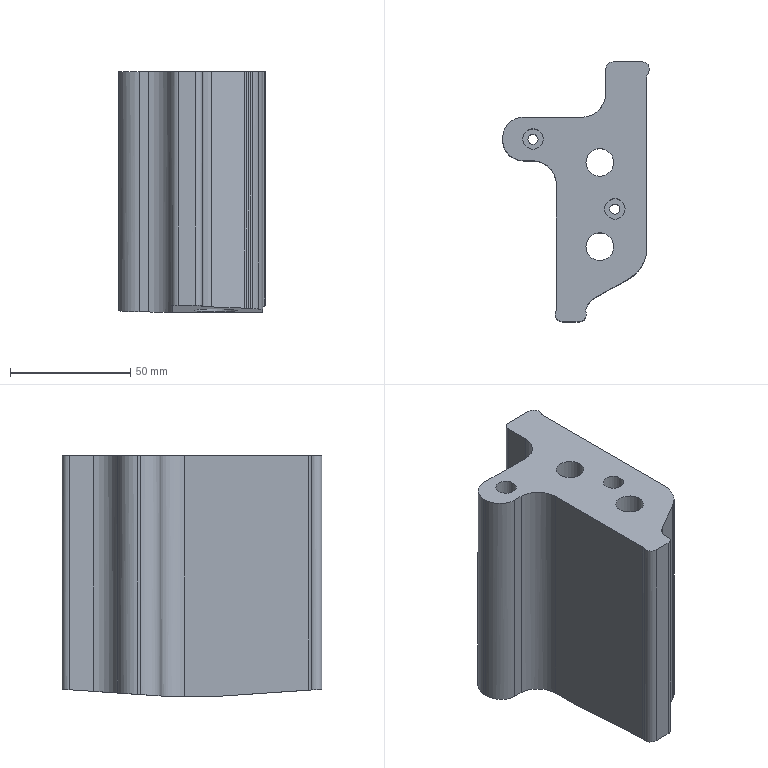Part | STEP file | lll_id250_x_t | 1 solid | 48 faces | box 60.865 x 107.859 x 100.003 mm | volume 310408 mm3 | cylinder 29 | plane 18 | cone 1 | commonest cylinder face diameters 6 x7 4.2 x2 8.506 x2 11.5 x2 17.001 x2 18.008 x2
STEP:
#1=CARTESIAN_POINT('',(449.,-109.43,-7.5));
#2=VERTEX_POINT('',#1);
#3=CARTESIAN_POINT('',(449.,-96.5,-7.5));
#4=VERTEX_POINT('',#3);
#5=CARTESIAN_POINT('',(449.,48.5,-7.5));
#6=DIRECTION('',(0.,1.,0.));
#7=VECTOR('',#6,1.);
#8=LINE('',#5,#7);
#9=EDGE_CURVE('',#2,#4,#8,.T.);
#10=ORIENTED_EDGE('',*,*,#9,.T.);
#11=CARTESIAN_POINT('',(446.115,-89.474,-7.502));
#12=VERTEX_POINT('',#11);
#13=CARTESIAN_POINT('',(438.999,-96.501,-7.5));
#14=DIRECTION('',(0.,0.,1.));
#15=DIRECTION('',(-1.,0.,0.));
#16=AXIS2_PLACEMENT_3D('',#13,#14,#15);
#17=CIRCLE('',#16,10.001);
#18=EDGE_CURVE('',#4,#12,#17,.T.);
#19=ORIENTED_EDGE('',*,*,#18,.T.);
#20=CARTESIAN_POINT('',(458.269,-89.43,-7.5));
#21=VERTEX_POINT('',#20);
#22=CARTESIAN_POINT('',(458.269,-89.43,-7.5));
#23=CARTESIAN_POINT('',(454.218,-89.444,-7.501));
#24=CARTESIAN_POINT('',(450.166,-89.459,-7.502));
#25=CARTESIAN_POINT('',(446.115,-89.474,-7.503));
#26=B_SPLINE_CURVE_WITH_KNOTS('',3,(#22,#23,#24,#25),.UNSPECIFIED.,.F.,.F.,(4,4),(0.,1.),.UNSPECIFIED.);
#27=EDGE_CURVE('',#21,#12,#26,.T.);
#28=ORIENTED_EDGE('',*,*,#27,.F.);
#29=CARTESIAN_POINT('',(475.731,-89.43,-7.5));
#30=VERTEX_POINT('',#29);
#31=CARTESIAN_POINT('',(467.,-87.231,-7.5));
#32=DIRECTION('',(0.,0.,-1.));
#33=DIRECTION('',(-1.,0.,0.));
#34=AXIS2_PLACEMENT_3D('',#31,#32,#33);
#35=CIRCLE('',#34,9.004);
#36=EDGE_CURVE('',#30,#21,#35,.T.);
#37=ORIENTED_EDGE('',*,*,#36,.F.);
#38=CARTESIAN_POINT('',(486.508,-89.43,-7.5));
#39=VERTEX_POINT('',#38);
#40=CARTESIAN_POINT('',(781.007,-89.43,-7.5));
#41=DIRECTION('',(-1.,0.,0.));
#42=VECTOR('',#41,1.);
#43=LINE('',#40,#42);
#44=EDGE_CURVE('',#39,#30,#43,.T.);
#45=ORIENTED_EDGE('',*,*,#44,.F.);
#46=CARTESIAN_POINT('',(486.507,-109.43,-7.5));
#47=VERTEX_POINT('',#46);
#48=CARTESIAN_POINT('',(486.516,48.518,-7.5));
#49=DIRECTION('',(-0.00006142,-1.,0.));
#50=VECTOR('',#49,1.);
#51=LINE('',#48,#50);
#52=EDGE_CURVE('',#39,#47,#51,.T.);
#53=ORIENTED_EDGE('',*,*,#52,.T.);
#54=CARTESIAN_POINT('',(465.982,-109.43,-7.5));
#55=VERTEX_POINT('',#54);
#56=CARTESIAN_POINT('',(488.085,-109.43,-7.5));
#57=DIRECTION('',(1.,0.,0.));
#58=VECTOR('',#57,1.);
#59=LINE('',#56,#58);
#60=EDGE_CURVE('',#55,#47,#59,.T.);
#61=ORIENTED_EDGE('',*,*,#60,.F.);
#62=CARTESIAN_POINT('',(458.045,-109.43,-7.5));
#63=VERTEX_POINT('',#62);
#64=CARTESIAN_POINT('',(462.014,-104.93,-7.5));
#65=DIRECTION('',(0.,0.,-1.));
#66=DIRECTION('',(-1.,0.,0.));
#67=AXIS2_PLACEMENT_3D('',#64,#65,#66);
#68=CIRCLE('',#67,6.);
#69=EDGE_CURVE('',#63,#55,#68,.T.);
#70=ORIENTED_EDGE('',*,*,#69,.F.);
#71=CARTESIAN_POINT('',(488.085,-109.43,-7.5));
#72=DIRECTION('',(1.,0.,0.));
#73=VECTOR('',#72,1.);
#74=LINE('',#71,#73);
#75=EDGE_CURVE('',#2,#63,#74,.T.);
#76=ORIENTED_EDGE('',*,*,#75,.F.);
#77=EDGE_LOOP('',(#10,#19,#28,#37,#45,#53,#61,#70,#76));
#78=FACE_BOUND('',#77,.T.);
#79=CARTESIAN_POINT('',(471.165,-106.5,-7.5));
#80=VERTEX_POINT('',#79);
#81=CARTESIAN_POINT('',(473.265,-106.5,-7.5));
#82=DIRECTION('',(0.,0.,1.));
#83=DIRECTION('',(-1.,0.,0.));
#84=AXIS2_PLACEMENT_3D('',#81,#82,#83);
#85=CIRCLE('',#84,2.1);
#86=EDGE_CURVE('',#80,#80,#85,.T.);
#87=ORIENTED_EDGE('',*,*,#86,.T.);
#88=EDGE_LOOP('',(#87));
#89=FACE_BOUND('',#88,.T.);
#90=CARTESIAN_POINT('',(781.007,48.5,-7.5));
#91=DIRECTION('',(0.,0.,-1.));
#92=DIRECTION('',(1.,0.,0.));
#93=AXIS2_PLACEMENT_3D('',#90,#91,#92);
#94=PLANE('',#93);
#95=ADVANCED_FACE('',(#78,#89),#94,.T.);
#96=CARTESIAN_POINT('',(476.004,-122.231,44.5));
#97=VERTEX_POINT('',#96);
#98=CARTESIAN_POINT('',(467.,-122.231,44.5));
#99=DIRECTION('',(0.,0.,-1.));
#100=DIRECTION('',(1.,0.,0.));
#101=AXIS2_PLACEMENT_3D('',#98,#99,#100);
#102=CIRCLE('',#101,9.004);
#103=EDGE_CURVE('',#97,#97,#102,.T.);
#104=ORIENTED_EDGE('',*,*,#103,.F.);
#105=EDGE_LOOP('',(#104));
#106=FACE_BOUND('',#105,.T.);
#107=CARTESIAN_POINT('',(467.,-131.235,-6.011));
#108=VERTEX_POINT('',#107);
#109=CARTESIAN_POINT('',(467.,-122.231,-6.626));
#110=DIRECTION('',(0.,-0.06813,-0.9977));
#111=DIRECTION('',(0.,-0.9977,0.06813));
#112=AXIS2_PLACEMENT_3D('',#109,#110,#111);
#113=ELLIPSE('',#112,9.025,9.004);
#114=EDGE_CURVE('',#108,#108,#113,.T.);
#115=ORIENTED_EDGE('',*,*,#114,.T.);
#116=EDGE_LOOP('',(#115));
#117=FACE_BOUND('',#116,.T.);
#118=CARTESIAN_POINT('',(467.,-122.231,-5.5));
#119=DIRECTION('',(0.,0.,1.));
#120=DIRECTION('',(1.,0.,0.));
#121=AXIS2_PLACEMENT_3D('',#118,#119,#120);
#122=CYLINDRICAL_SURFACE('',#121,9.004);
#123=ADVANCED_FACE('',(#106,#117),#122,.F.);
#124=CARTESIAN_POINT('',(468.014,-104.93,-2.296));
#125=VERTEX_POINT('',#124);
#126=CARTESIAN_POINT('',(462.014,-104.93,-2.296));
#127=DIRECTION('',(0.,0.,1.));
#128=DIRECTION('',(1.,0.,0.));
#129=AXIS2_PLACEMENT_3D('',#126,#127,#128);
#130=CIRCLE('',#129,6.);
#131=EDGE_CURVE('',#125,#125,#130,.T.);
#132=ORIENTED_EDGE('',*,*,#131,.T.);
#133=EDGE_LOOP('',(#132));
#134=FACE_BOUND('',#133,.T.);
#135=CARTESIAN_POINT('',(462.014,-104.93,-7.807));
#136=DIRECTION('',(0.,-0.06813,-0.9977));
#137=DIRECTION('',(0.,-0.9977,0.06813));
#138=AXIS2_PLACEMENT_3D('',#135,#136,#137);
#139=ELLIPSE('',#138,6.014,6.);
#140=EDGE_CURVE('',#55,#63,#139,.T.);
#141=ORIENTED_EDGE('',*,*,#140,.T.);
#142=ORIENTED_EDGE('',*,*,#69,.T.);
#143=EDGE_LOOP('',(#141,#142));
#144=FACE_BOUND('',#143,.T.);
#145=CARTESIAN_POINT('',(462.014,-104.93,-7.296));
#146=DIRECTION('',(0.,0.,1.));
#147=DIRECTION('',(-1.,0.,0.));
#148=AXIS2_PLACEMENT_3D('',#145,#146,#147);
#149=CYLINDRICAL_SURFACE('',#148,6.);
#150=ADVANCED_FACE('',(#134,#144),#149,.F.);
#151=ORIENTED_EDGE('',*,*,#103,.T.);
#152=EDGE_LOOP('',(#151));
#153=FACE_BOUND('',#152,.T.);
#154=CARTESIAN_POINT('',(472.75,-122.231,44.5));
#155=VERTEX_POINT('',#154);
#156=CARTESIAN_POINT('',(467.,-122.231,44.5));
#157=DIRECTION('',(0.,0.,1.));
#158=DIRECTION('',(1.,0.,0.));
#159=AXIS2_PLACEMENT_3D('',#156,#157,#158);
#160=CIRCLE('',#159,5.75);
#161=EDGE_CURVE('',#155,#155,#160,.T.);
#162=ORIENTED_EDGE('',*,*,#161,.T.);
#163=EDGE_LOOP('',(#162));
#164=FACE_BOUND('',#163,.T.);
#165=CARTESIAN_POINT('',(467.,-122.231,44.5));
#166=DIRECTION('',(0.,0.,1.));
#167=DIRECTION('',(1.,0.,0.));
#168=AXIS2_PLACEMENT_3D('',#165,#166,#167);
#169=PLANE('',#168);
#170=ADVANCED_FACE('',(#153,#164),#169,.F.);
#171=CARTESIAN_POINT('',(476.004,-87.231,44.5));
#172=VERTEX_POINT('',#171);
#173=CARTESIAN_POINT('',(467.,-87.231,44.5));
#174=DIRECTION('',(0.,0.,-1.));
#175=DIRECTION('',(1.,0.,0.));
#176=AXIS2_PLACEMENT_3D('',#173,#174,#175);
#177=CIRCLE('',#176,9.004);
#178=EDGE_CURVE('',#172,#172,#177,.T.);
#179=ORIENTED_EDGE('',*,*,#178,.T.);
#180=EDGE_LOOP('',(#179));
#181=FACE_BOUND('',#180,.T.);
#182=CARTESIAN_POINT('',(472.75,-87.231,44.5));
#183=VERTEX_POINT('',#182);
#184=CARTESIAN_POINT('',(467.,-87.231,44.5));
#185=DIRECTION('',(0.,0.,1.));
#186=DIRECTION('',(1.,0.,0.));
#187=AXIS2_PLACEMENT_3D('',#184,#185,#186);
#188=CIRCLE('',#187,5.75);
#189=EDGE_CURVE('',#183,#183,#188,.T.);
#190=ORIENTED_EDGE('',*,*,#189,.T.);
#191=EDGE_LOOP('',(#190));
#192=FACE_BOUND('',#191,.T.);
#193=CARTESIAN_POINT('',(467.,-87.231,44.5));
#194=DIRECTION('',(0.,0.,1.));
#195=DIRECTION('',(1.,0.,0.));
#196=AXIS2_PLACEMENT_3D('',#193,#194,#195);
#197=PLANE('',#196);
#198=ADVANCED_FACE('',(#181,#192),#197,.F.);
#199=CARTESIAN_POINT('',(469.012,-106.5,30.747));
#200=VERTEX_POINT('',#199);
#201=CARTESIAN_POINT('',(473.265,-106.5,30.747));
#202=DIRECTION('',(0.,0.,1.));
#203=DIRECTION('',(-1.,0.,0.));
#204=AXIS2_PLACEMENT_3D('',#201,#202,#203);
#205=CIRCLE('',#204,4.253);
#206=EDGE_CURVE('',#200,#200,#205,.T.);
#207=ORIENTED_EDGE('',*,*,#206,.F.);
#208=EDGE_LOOP('',(#207));
#209=FACE_BOUND('',#208,.T.);
#210=CARTESIAN_POINT('',(469.012,-106.5,92.5));
#211=VERTEX_POINT('',#210);
#212=CARTESIAN_POINT('',(473.265,-106.5,92.5));
#213=DIRECTION('',(0.,0.,-1.));
#214=DIRECTION('',(-1.,0.,0.));
#215=AXIS2_PLACEMENT_3D('',#212,#213,#214);
#216=CIRCLE('',#215,4.253);
#217=EDGE_CURVE('',#211,#211,#216,.T.);
#218=ORIENTED_EDGE('',*,*,#217,.F.);
#219=EDGE_LOOP('',(#218));
#220=FACE_BOUND('',#219,.T.);
#221=CARTESIAN_POINT('',(473.265,-106.5,180.747));
#222=DIRECTION('',(0.,0.,-1.));
#223=DIRECTION('',(1.,0.,0.));
#224=AXIS2_PLACEMENT_3D('',#221,#222,#223);
#225=CYLINDRICAL_SURFACE('',#224,4.253);
#226=ADVANCED_FACE('',(#209,#220),#225,.F.);
#227=CARTESIAN_POINT('',(435.012,-77.5,30.747));
#228=VERTEX_POINT('',#227);
#229=CARTESIAN_POINT('',(439.265,-77.5,30.747));
#230=DIRECTION('',(0.,0.,1.));
#231=DIRECTION('',(-1.,0.,0.));
#232=AXIS2_PLACEMENT_3D('',#229,#230,#231);
#233=CIRCLE('',#232,4.253);
#234=EDGE_CURVE('',#228,#228,#233,.T.);
#235=ORIENTED_EDGE('',*,*,#234,.F.);
#236=EDGE_LOOP('',(#235));
#237=FACE_BOUND('',#236,.T.);
#238=CARTESIAN_POINT('',(435.012,-77.5,92.5));
#239=VERTEX_POINT('',#238);
#240=CARTESIAN_POINT('',(439.265,-77.5,92.5));
#241=DIRECTION('',(0.,0.,-1.));
#242=DIRECTION('',(-1.,0.,0.));
#243=AXIS2_PLACEMENT_3D('',#240,#241,#242);
#244=CIRCLE('',#243,4.253);
#245=EDGE_CURVE('',#239,#239,#244,.T.);
#246=ORIENTED_EDGE('',*,*,#245,.F.);
#247=EDGE_LOOP('',(#246));
#248=FACE_BOUND('',#247,.T.);
#249=CARTESIAN_POINT('',(439.265,-77.5,180.747));
#250=DIRECTION('',(0.,0.,-1.));
#251=DIRECTION('',(1.,0.,0.));
#252=AXIS2_PLACEMENT_3D('',#249,#250,#251);
#253=CYLINDRICAL_SURFACE('',#252,4.253);
#254=ADVANCED_FACE('',(#237,#248),#253,.F.);
#255=CARTESIAN_POINT('',(471.165,-106.5,30.747));
#256=VERTEX_POINT('',#255);
#257=CARTESIAN_POINT('',(473.265,-106.5,30.747));
#258=DIRECTION('',(0.,0.,1.));
#259=DIRECTION('',(-1.,0.,0.));
#260=AXIS2_PLACEMENT_3D('',#257,#258,#259);
#261=CIRCLE('',#260,2.1);
#262=EDGE_CURVE('',#256,#256,#261,.T.);
#263=ORIENTED_EDGE('',*,*,#262,.F.);
#264=EDGE_LOOP('',(#263));
#265=FACE_BOUND('',#264,.T.);
#266=ORIENTED_EDGE('',*,*,#206,.T.);
#267=EDGE_LOOP('',(#266));
#268=FACE_BOUND('',#267,.T.);
#269=CARTESIAN_POINT('',(473.265,-106.5,30.747));
#270=DIRECTION('',(0.,0.,-1.));
#271=DIRECTION('',(1.,0.,0.));
#272=AXIS2_PLACEMENT_3D('',#269,#270,#271);
#273=PLANE('',#272);
#274=ADVANCED_FACE('',(#265,#268),#273,.F.);
#275=ORIENTED_EDGE('',*,*,#262,.T.);
#276=EDGE_LOOP('',(#275));
#277=FACE_BOUND('',#276,.T.);
#278=ORIENTED_EDGE('',*,*,#86,.F.);
#279=EDGE_LOOP('',(#278));
#280=FACE_BOUND('',#279,.T.);
#281=CARTESIAN_POINT('',(473.265,-106.5,1343.726));
#282=DIRECTION('',(0.,0.,-1.));
#283=DIRECTION('',(1.,0.,0.));
#284=AXIS2_PLACEMENT_3D('',#281,#282,#283);
#285=CYLINDRICAL_SURFACE('',#284,2.1);
#286=ADVANCED_FACE('',(#277,#280),#285,.F.);
#287=CARTESIAN_POINT('',(437.165,-77.5,30.747));
#288=VERTEX_POINT('',#287);
#289=CARTESIAN_POINT('',(439.265,-77.5,30.747));
#290=DIRECTION('',(0.,0.,1.));
#291=DIRECTION('',(-1.,0.,0.));
#292=AXIS2_PLACEMENT_3D('',#289,#290,#291);
#293=CIRCLE('',#292,2.1);
#294=EDGE_CURVE('',#288,#288,#293,.T.);
#295=ORIENTED_EDGE('',*,*,#294,.F.);
#296=EDGE_LOOP('',(#295));
#297=FACE_BOUND('',#296,.T.);
#298=ORIENTED_EDGE('',*,*,#234,.T.);
#299=EDGE_LOOP('',(#298));
#300=FACE_BOUND('',#299,.T.);
#301=CARTESIAN_POINT('',(439.265,-77.5,30.747));
#302=DIRECTION('',(0.,0.,-1.));
#303=DIRECTION('',(1.,0.,0.));
#304=AXIS2_PLACEMENT_3D('',#301,#302,#303);
#305=PLANE('',#304);
#306=ADVANCED_FACE('',(#297,#300),#305,.F.);
#307=CARTESIAN_POINT('',(439.265,-79.6,-6.829));
#308=VERTEX_POINT('',#307);
#309=CARTESIAN_POINT('',(439.265,-77.5,-6.685));
#310=DIRECTION('',(0.,-0.06813,0.9977));
#311=DIRECTION('',(0.,-0.9977,-0.06813));
#312=AXIS2_PLACEMENT_3D('',#309,#310,#311);
#313=ELLIPSE('',#312,2.105,2.1);
#314=EDGE_CURVE('',#308,#308,#313,.T.);
#315=ORIENTED_EDGE('',*,*,#314,.F.);
#316=EDGE_LOOP('',(#315));
#317=FACE_BOUND('',#316,.T.);
#318=ORIENTED_EDGE('',*,*,#294,.T.);
#319=EDGE_LOOP('',(#318));
#320=FACE_BOUND('',#319,.T.);
#321=CARTESIAN_POINT('',(439.265,-77.5,1343.726));
#322=DIRECTION('',(0.,0.,-1.));
#323=DIRECTION('',(1.,0.,0.));
#324=AXIS2_PLACEMENT_3D('',#321,#322,#323);
#325=CYLINDRICAL_SURFACE('',#324,2.1);
#326=ADVANCED_FACE('',(#317,#320),#325,.F.);
#327=ORIENTED_EDGE('',*,*,#36,.T.);
#328=CARTESIAN_POINT('',(467.,-87.231,-7.35));
#329=DIRECTION('',(0.,-0.06813,0.9977));
#330=DIRECTION('',(0.,0.9977,0.06813));
#331=AXIS2_PLACEMENT_3D('',#328,#329,#330);
#332=ELLIPSE('',#331,9.025,9.004);
#333=EDGE_CURVE('',#30,#21,#332,.T.);
#334=ORIENTED_EDGE('',*,*,#333,.F.);
#335=EDGE_LOOP('',(#327,#334));
#336=FACE_BOUND('',#335,.T.);
#337=ORIENTED_EDGE('',*,*,#178,.F.);
#338=EDGE_LOOP('',(#337));
#339=FACE_BOUND('',#338,.T.);
#340=CARTESIAN_POINT('',(467.,-87.231,-5.5));
#341=DIRECTION('',(0.,0.,1.));
#342=DIRECTION('',(1.,0.,0.));
#343=AXIS2_PLACEMENT_3D('',#340,#341,#342);
#344=CYLINDRICAL_SURFACE('',#343,9.004);
#345=ADVANCED_FACE('',(#336,#339),#344,.F.);
#346=ORIENTED_EDGE('',*,*,#161,.F.);
#347=EDGE_LOOP('',(#346));
#348=FACE_BOUND('',#347,.T.);
#349=CARTESIAN_POINT('',(461.25,-122.231,92.5));
#350=VERTEX_POINT('',#349);
#351=CARTESIAN_POINT('',(467.,-122.231,92.5));
#352=DIRECTION('',(0.,0.,-1.));
#353=DIRECTION('',(-1.,0.,0.));
#354=AXIS2_PLACEMENT_3D('',#351,#352,#353);
#355=CIRCLE('',#354,5.75);
#356=EDGE_CURVE('',#350,#350,#355,.T.);
#357=ORIENTED_EDGE('',*,*,#356,.F.);
#358=EDGE_LOOP('',(#357));
#359=FACE_BOUND('',#358,.T.);
#360=CARTESIAN_POINT('',(467.,-122.231,94.5));
#361=DIRECTION('',(0.,0.,-1.));
#362=DIRECTION('',(1.,0.,0.));
#363=AXIS2_PLACEMENT_3D('',#360,#361,#362);
#364=CYLINDRICAL_SURFACE('',#363,5.75);
#365=ADVANCED_FACE('',(#348,#359),#364,.F.);
#366=CARTESIAN_POINT('',(461.302,-149.551,92.5));
#367=VERTEX_POINT('',#366);
#368=CARTESIAN_POINT('',(461.369,-147.727,92.5));
#369=VERTEX_POINT('',#368);
#370=CARTESIAN_POINT('',(464.191,-148.744,92.5));
#371=DIRECTION('',(0.,0.,-1.));
#372=DIRECTION('',(-1.,0.,0.));
#373=AXIS2_PLACEMENT_3D('',#370,#371,#372);
#374=CIRCLE('',#373,3.);
#375=EDGE_CURVE('',#367,#369,#374,.T.);
#376=ORIENTED_EDGE('',*,*,#375,.T.);
#377=CARTESIAN_POINT('',(465.269,-143.286,92.5));
#378=VERTEX_POINT('',#377);
#379=CARTESIAN_POINT('',(468.962,-150.461,92.5));
#380=DIRECTION('',(0.,0.,-1.));
#381=DIRECTION('',(-1.,0.,0.));
#382=AXIS2_PLACEMENT_3D('',#379,#380,#381);
#383=CIRCLE('',#382,8.07);
#384=EDGE_CURVE('',#369,#378,#383,.T.);
#385=ORIENTED_EDGE('',*,*,#384,.T.);
#386=CARTESIAN_POINT('',(478.829,-135.663,92.5));
#387=VERTEX_POINT('',#386);
#388=CARTESIAN_POINT('',(455.316,-148.881,92.5));
#389=DIRECTION('',(0.8717,0.49,0.));
#390=VECTOR('',#389,1.);
#391=LINE('',#388,#390);
#392=EDGE_CURVE('',#378,#387,#391,.T.);
#393=ORIENTED_EDGE('',*,*,#392,.T.);
#394=CARTESIAN_POINT('',(479.654,-135.117,92.5));
#395=VERTEX_POINT('',#394);
#396=CARTESIAN_POINT('',(448.181,-88.407,92.5));
#397=DIRECTION('',(0.,0.,1.));
#398=DIRECTION('',(-1.,0.,0.));
#399=AXIS2_PLACEMENT_3D('',#396,#397,#398);
#400=CIRCLE('',#399,56.324);
#401=EDGE_CURVE('',#387,#395,#400,.T.);
#402=ORIENTED_EDGE('',*,*,#401,.T.);
#403=CARTESIAN_POINT('',(480.466,-134.556,92.5));
#404=VERTEX_POINT('',#403);
#405=CARTESIAN_POINT('',(462.354,-109.242,92.5));
#406=DIRECTION('',(0.,0.,1.));
#407=DIRECTION('',(-1.,0.,0.));
#408=AXIS2_PLACEMENT_3D('',#405,#406,#407);
#409=CIRCLE('',#408,31.126);
#410=EDGE_CURVE('',#395,#404,#409,.T.);
#411=ORIENTED_EDGE('',*,*,#410,.T.);
#412=CARTESIAN_POINT('',(481.25,-133.962,92.5));
#413=VERTEX_POINT('',#412);
#414=CARTESIAN_POINT('',(469.718,-119.534,92.5));
#415=DIRECTION('',(0.,0.,1.));
#416=DIRECTION('',(-1.,0.,0.));
#417=AXIS2_PLACEMENT_3D('',#414,#415,#416);
#418=CIRCLE('',#417,18.471);
#419=EDGE_CURVE('',#404,#413,#418,.T.);
#420=ORIENTED_EDGE('',*,*,#419,.T.);
#421=CARTESIAN_POINT('',(482.171,-133.152,92.5));
#422=VERTEX_POINT('',#421);
#423=CARTESIAN_POINT('',(473.427,-124.145,92.5));
#424=DIRECTION('',(0.,0.,-1.));
#425=DIRECTION('',(-1.,0.,0.));
#426=AXIS2_PLACEMENT_3D('',#423,#424,#425);
#427=CIRCLE('',#426,12.553);
#428=EDGE_CURVE('',#422,#413,#427,.T.);
#429=ORIENTED_EDGE('',*,*,#428,.F.);
#430=CARTESIAN_POINT('',(484.678,-129.804,92.5));
#431=VERTEX_POINT('',#430);
#432=CARTESIAN_POINT('',(472.01,-122.929,92.5));
#433=DIRECTION('',(0.,0.,-1.));
#434=DIRECTION('',(-1.,0.,0.));
#435=AXIS2_PLACEMENT_3D('',#432,#433,#434);
#436=CIRCLE('',#435,14.414);
#437=EDGE_CURVE('',#431,#422,#436,.T.);
#438=ORIENTED_EDGE('',*,*,#437,.F.);
#439=CARTESIAN_POINT('',(486.461,-123.716,92.5));
#440=VERTEX_POINT('',#439);
#441=CARTESIAN_POINT('',(472.347,-122.889,92.5));
#442=DIRECTION('',(0.,0.,-1.));
#443=DIRECTION('',(-1.,0.,0.));
#444=AXIS2_PLACEMENT_3D('',#441,#442,#443);
#445=CIRCLE('',#444,14.138);
#446=EDGE_CURVE('',#440,#431,#445,.T.);
#447=ORIENTED_EDGE('',*,*,#446,.F.);
#448=CARTESIAN_POINT('',(486.506,-122.731,92.5));
#449=VERTEX_POINT('',#448);
#450=CARTESIAN_POINT('',(439.156,-121.059,92.5));
#451=DIRECTION('',(0.,0.,-1.));
#452=DIRECTION('',(-1.,0.,0.));
#453=AXIS2_PLACEMENT_3D('',#450,#451,#452);
#454=CIRCLE('',#453,47.38);
#455=EDGE_CURVE('',#449,#440,#454,.T.);
#456=ORIENTED_EDGE('',*,*,#455,.F.);
#457=CARTESIAN_POINT('',(486.51,-51.898,92.5));
#458=VERTEX_POINT('',#457);
#459=CARTESIAN_POINT('',(486.506,-121.062,92.5));
#460=DIRECTION('',(0.00006142,1.,0.));
#461=VECTOR('',#460,1.);
#462=LINE('',#459,#461);
#463=EDGE_CURVE('',#449,#458,#462,.T.);
#464=ORIENTED_EDGE('',*,*,#463,.T.);
#465=CARTESIAN_POINT('',(487.038,-50.199,92.5));
#466=VERTEX_POINT('',#465);
#467=CARTESIAN_POINT('',(489.51,-51.898,92.5));
#468=DIRECTION('',(0.,0.,-1.));
#469=DIRECTION('',(-1.,0.,0.));
#470=AXIS2_PLACEMENT_3D('',#467,#468,#469);
#471=CIRCLE('',#470,3.);
#472=EDGE_CURVE('',#458,#466,#471,.T.);
#473=ORIENTED_EDGE('',*,*,#472,.T.);
#474=CARTESIAN_POINT('',(484.565,-45.5,92.5));
#475=VERTEX_POINT('',#474);
#476=CARTESIAN_POINT('',(484.565,-48.5,92.5));
#477=DIRECTION('',(0.,0.,1.));
#478=DIRECTION('',(-1.,0.,0.));
#479=AXIS2_PLACEMENT_3D('',#476,#477,#478);
#480=CIRCLE('',#479,3.);
#481=EDGE_CURVE('',#466,#475,#480,.T.);
#482=ORIENTED_EDGE('',*,*,#481,.T.);
#483=CARTESIAN_POINT('',(472.5,-45.5,92.5));
#484=VERTEX_POINT('',#483);
#485=CARTESIAN_POINT('',(439.676,-45.5,92.5));
#486=DIRECTION('',(1.,0.,0.));
#487=VECTOR('',#486,1.);
#488=LINE('',#485,#487);
#489=EDGE_CURVE('',#484,#475,#488,.T.);
#490=ORIENTED_EDGE('',*,*,#489,.F.);
#491=CARTESIAN_POINT('',(469.5,-48.5,92.5));
#492=VERTEX_POINT('',#491);
#493=CARTESIAN_POINT('',(472.5,-48.5,92.5));
#494=DIRECTION('',(0.,0.,-1.));
#495=DIRECTION('',(-1.,0.,0.));
#496=AXIS2_PLACEMENT_3D('',#493,#494,#495);
#497=CIRCLE('',#496,3.);
#498=EDGE_CURVE('',#492,#484,#497,.T.);
#499=ORIENTED_EDGE('',*,*,#498,.F.);
#500=CARTESIAN_POINT('',(469.5,-58.5,92.5));
#501=VERTEX_POINT('',#500);
#502=CARTESIAN_POINT('',(469.5,-121.059,92.5));
#503=DIRECTION('',(0.,1.,0.));
#504=VECTOR('',#503,1.);
#505=LINE('',#502,#504);
#506=EDGE_CURVE('',#501,#492,#505,.T.);
#507=ORIENTED_EDGE('',*,*,#506,.F.);
#508=CARTESIAN_POINT('',(459.5,-68.5,92.5));
#509=VERTEX_POINT('',#508);
#510=CARTESIAN_POINT('',(459.499,-58.499,92.5));
#511=DIRECTION('',(0.,0.,1.));
#512=DIRECTION('',(-1.,0.,0.));
#513=AXIS2_PLACEMENT_3D('',#510,#511,#512);
#514=CIRCLE('',#513,10.001);
#515=EDGE_CURVE('',#509,#501,#514,.T.);
#516=ORIENTED_EDGE('',*,*,#515,.F.);
#517=CARTESIAN_POINT('',(435.2,-68.5,92.5));
#518=VERTEX_POINT('',#517);
#519=CARTESIAN_POINT('',(439.676,-68.5,92.5));
#520=DIRECTION('',(-1.,0.,0.));
#521=VECTOR('',#520,1.);
#522=LINE('',#519,#521);
#523=EDGE_CURVE('',#509,#518,#522,.T.);
#524=ORIENTED_EDGE('',*,*,#523,.T.);
#525=CARTESIAN_POINT('',(426.7,-77.,92.5));
#526=VERTEX_POINT('',#525);
#527=CARTESIAN_POINT('',(435.2,-77.,92.5));
#528=DIRECTION('',(0.,0.,1.));
#529=DIRECTION('',(-1.,0.,0.));
#530=AXIS2_PLACEMENT_3D('',#527,#528,#529);
#531=CIRCLE('',#530,8.5);
#532=EDGE_CURVE('',#518,#526,#531,.T.);
#533=ORIENTED_EDGE('',*,*,#532,.T.);
#534=CARTESIAN_POINT('',(426.7,-78.,92.5));
#535=VERTEX_POINT('',#534);
#536=CARTESIAN_POINT('',(426.7,-121.059,92.5));
#537=DIRECTION('',(0.,-1.,0.));
#538=VECTOR('',#537,1.);
#539=LINE('',#536,#538);
#540=EDGE_CURVE('',#526,#535,#539,.T.);
#541=ORIENTED_EDGE('',*,*,#540,.T.);
#542=CARTESIAN_POINT('',(435.2,-86.5,92.5));
#543=VERTEX_POINT('',#542);
#544=CARTESIAN_POINT('',(435.2,-78.,92.5));
#545=DIRECTION('',(0.,0.,1.));
#546=DIRECTION('',(-1.,0.,0.));
#547=AXIS2_PLACEMENT_3D('',#544,#545,#546);
#548=CIRCLE('',#547,8.5);
#549=EDGE_CURVE('',#535,#543,#548,.T.);
#550=ORIENTED_EDGE('',*,*,#549,.T.);
#551=CARTESIAN_POINT('',(439.,-86.5,92.5));
#552=VERTEX_POINT('',#551);
#553=CARTESIAN_POINT('',(439.676,-86.5,92.5));
#554=DIRECTION('',(-1.,0.,0.));
#555=VECTOR('',#554,1.);
#556=LINE('',#553,#555);
#557=EDGE_CURVE('',#552,#543,#556,.T.);
#558=ORIENTED_EDGE('',*,*,#557,.F.);
#559=CARTESIAN_POINT('',(449.,-96.5,92.5));
#560=VERTEX_POINT('',#559);
#561=CARTESIAN_POINT('',(438.999,-96.501,92.5));
#562=DIRECTION('',(0.,0.,-1.));
#563=DIRECTION('',(-1.,0.,0.));
#564=AXIS2_PLACEMENT_3D('',#561,#562,#563);
#565=CIRCLE('',#564,10.001);
#566=EDGE_CURVE('',#552,#560,#565,.T.);
#567=ORIENTED_EDGE('',*,*,#566,.T.);
#568=CARTESIAN_POINT('',(449.,-147.961,92.5));
#569=VERTEX_POINT('',#568);
#570=CARTESIAN_POINT('',(449.,-121.059,92.5));
#571=DIRECTION('',(0.,1.,0.));
#572=VECTOR('',#571,1.);
#573=LINE('',#570,#572);
#574=EDGE_CURVE('',#569,#560,#573,.T.);
#575=ORIENTED_EDGE('',*,*,#574,.F.);
#576=CARTESIAN_POINT('',(448.75,-149.16,92.5));
#577=VERTEX_POINT('',#576);
#578=CARTESIAN_POINT('',(446.,-147.961,92.5));
#579=DIRECTION('',(0.,0.,-1.));
#580=DIRECTION('',(-1.,0.,0.));
#581=AXIS2_PLACEMENT_3D('',#578,#579,#580);
#582=CIRCLE('',#581,3.);
#583=EDGE_CURVE('',#569,#577,#582,.T.);
#584=ORIENTED_EDGE('',*,*,#583,.T.);
#585=CARTESIAN_POINT('',(451.5,-153.359,92.5));
#586=VERTEX_POINT('',#585);
#587=CARTESIAN_POINT('',(451.5,-150.359,92.5));
#588=DIRECTION('',(0.,0.,1.));
#589=DIRECTION('',(-1.,0.,0.));
#590=AXIS2_PLACEMENT_3D('',#587,#588,#589);
#591=CIRCLE('',#590,3.);
#592=EDGE_CURVE('',#577,#586,#591,.T.);
#593=ORIENTED_EDGE('',*,*,#592,.T.);
#594=CARTESIAN_POINT('',(458.413,-153.359,92.5));
#595=VERTEX_POINT('',#594);
#596=CARTESIAN_POINT('',(439.676,-153.359,92.5));
#597=DIRECTION('',(1.,0.,0.));
#598=VECTOR('',#597,1.);
#599=LINE('',#596,#598);
#600=EDGE_CURVE('',#586,#595,#599,.T.);
#601=ORIENTED_EDGE('',*,*,#600,.T.);
#602=CARTESIAN_POINT('',(458.413,-150.359,92.5));
#603=DIRECTION('',(0.,0.,-1.));
#604=DIRECTION('',(-1.,0.,0.));
#605=AXIS2_PLACEMENT_3D('',#602,#603,#604);
#606=CIRCLE('',#605,3.);
#607=EDGE_CURVE('',#367,#595,#606,.T.);
#608=ORIENTED_EDGE('',*,*,#607,.F.);
#609=EDGE_LOOP('',(#376,#385,#393,#402,#411,#420,#429,#438,#447,#456,#464,#473,#482,#490,#499,#507,#516,#524,#533,#541,#550,#558,#567,#575,#584,#593,#601,#608));
#610=FACE_BOUND('',#609,.T.);
#611=ORIENTED_EDGE('',*,*,#245,.T.);
#612=EDGE_LOOP('',(#611));
#613=FACE_BOUND('',#612,.T.);
#614=ORIENTED_EDGE('',*,*,#217,.T.);
#615=EDGE_LOOP('',(#614));
#616=FACE_BOUND('',#615,.T.);
#617=ORIENTED_EDGE('',*,*,#356,.T.);
#618=EDGE_LOOP('',(#617));
#619=FACE_BOUND('',#618,.T.);
#620=CARTESIAN_POINT('',(461.25,-87.231,92.5));
#621=VERTEX_POINT('',#620);
#622=CARTESIAN_POINT('',(467.,-87.231,92.5));
#623=DIRECTION('',(0.,0.,-1.));
#624=DIRECTION('',(-1.,0.,0.));
#625=AXIS2_PLACEMENT_3D('',#622,#623,#624);
#626=CIRCLE('',#625,5.75);
#627=EDGE_CURVE('',#621,#621,#626,.T.);
#628=ORIENTED_EDGE('',*,*,#627,.T.);
#629=EDGE_LOOP('',(#628));
#630=FACE_BOUND('',#629,.T.);
#631=CARTESIAN_POINT('',(439.676,-121.059,92.5));
#632=DIRECTION('',(0.,0.,-1.));
#633=DIRECTION('',(1.,0.,0.));
#634=AXIS2_PLACEMENT_3D('',#631,#632,#633);
#635=PLANE('',#634);
#636=ADVANCED_FACE('',(#610,#613,#616,#619,#630),#635,.F.);
#637=ORIENTED_EDGE('',*,*,#189,.F.);
#638=EDGE_LOOP('',(#637));
#639=FACE_BOUND('',#638,.T.);
#640=ORIENTED_EDGE('',*,*,#627,.F.);
#641=EDGE_LOOP('',(#640));
#642=FACE_BOUND('',#641,.T.);
#643=CARTESIAN_POINT('',(467.,-87.231,94.5));
#644=DIRECTION('',(0.,0.,-1.));
#645=DIRECTION('',(1.,0.,0.));
#646=AXIS2_PLACEMENT_3D('',#643,#644,#645);
#647=CYLINDRICAL_SURFACE('',#646,5.75);
#648=ADVANCED_FACE('',(#639,#642),#647,.F.);
#649=ORIENTED_EDGE('',*,*,#131,.F.);
#650=EDGE_LOOP('',(#649));
#651=FACE_BOUND('',#650,.T.);
#652=CARTESIAN_POINT('',(466.266,-104.93,-2.296));
#653=VERTEX_POINT('',#652);
#654=CARTESIAN_POINT('',(462.014,-104.93,-2.296));
#655=DIRECTION('',(0.,0.,-1.));
#656=DIRECTION('',(1.,0.,0.));
#657=AXIS2_PLACEMENT_3D('',#654,#655,#656);
#658=CIRCLE('',#657,4.253);
#659=EDGE_CURVE('',#653,#653,#658,.T.);
#660=ORIENTED_EDGE('',*,*,#659,.F.);
#661=EDGE_LOOP('',(#660));
#662=FACE_BOUND('',#661,.T.);
#663=CARTESIAN_POINT('',(462.014,-104.93,-2.296));
#664=DIRECTION('',(0.,0.,1.));
#665=DIRECTION('',(-1.,0.,0.));
#666=AXIS2_PLACEMENT_3D('',#663,#664,#665);
#667=PLANE('',#666);
#668=ADVANCED_FACE('',(#651,#662),#667,.F.);
#669=CARTESIAN_POINT('',(462.014,-104.93,27.506));
#670=VERTEX_POINT('',#669);
#671=VERTEX_LOOP('',#670);
#672=FACE_BOUND('',#671,.T.);
#673=CARTESIAN_POINT('',(466.266,-104.93,23.253));
#674=VERTEX_POINT('',#673);
#675=CARTESIAN_POINT('',(462.014,-104.93,23.253));
#676=DIRECTION('',(0.,0.,1.));
#677=DIRECTION('',(1.,0.,0.));
#678=AXIS2_PLACEMENT_3D('',#675,#676,#677);
#679=CIRCLE('',#678,4.253);
#680=EDGE_CURVE('',#674,#674,#679,.T.);
#681=ORIENTED_EDGE('',*,*,#680,.F.);
#682=EDGE_LOOP('',(#681));
#683=FACE_BOUND('',#682,.T.);
#684=CARTESIAN_POINT('',(462.014,-104.93,23.253));
#685=DIRECTION('',(0.,0.,-1.));
#686=DIRECTION('',(1.,0.,0.));
#687=AXIS2_PLACEMENT_3D('',#684,#685,#686);
#688=CONICAL_SURFACE('',#687,4.253,45.);
#689=ADVANCED_FACE('',(#672,#683),#688,.F.);
#690=ORIENTED_EDGE('',*,*,#659,.T.);
#691=EDGE_LOOP('',(#690));
#692=FACE_BOUND('',#691,.T.);
#693=ORIENTED_EDGE('',*,*,#680,.T.);
#694=EDGE_LOOP('',(#693));
#695=FACE_BOUND('',#694,.T.);
#696=CARTESIAN_POINT('',(462.014,-104.93,-7.5));
#697=DIRECTION('',(0.,0.,1.));
#698=DIRECTION('',(-1.,0.,0.));
#699=AXIS2_PLACEMENT_3D('',#696,#697,#698);
#700=CYLINDRICAL_SURFACE('',#699,4.253);
#701=ADVANCED_FACE('',(#692,#695),#700,.F.);
#702=ORIENTED_EDGE('',*,*,#314,.T.);
#703=EDGE_LOOP('',(#702));
#704=FACE_BOUND('',#703,.T.);
#705=ORIENTED_EDGE('',*,*,#27,.T.);
#706=CARTESIAN_POINT('',(439.,-86.5,-7.3));
#707=VERTEX_POINT('',#706);
#708=CARTESIAN_POINT('',(438.999,-96.501,-7.983));
#709=DIRECTION('',(0.,0.06813,-0.9977));
#710=DIRECTION('',(0.,0.9977,0.06813));
#711=AXIS2_PLACEMENT_3D('',#708,#709,#710);
#712=ELLIPSE('',#711,10.024,10.001);
#713=EDGE_CURVE('',#707,#12,#712,.T.);
#714=ORIENTED_EDGE('',*,*,#713,.F.);
#715=CARTESIAN_POINT('',(435.2,-86.5,-7.3));
#716=VERTEX_POINT('',#715);
#717=CARTESIAN_POINT('',(488.085,-86.5,-7.3));
#718=DIRECTION('',(1.,0.,0.));
#719=VECTOR('',#718,1.);
#720=LINE('',#717,#719);
#721=EDGE_CURVE('',#716,#707,#720,.T.);
#722=ORIENTED_EDGE('',*,*,#721,.F.);
#723=CARTESIAN_POINT('',(426.7,-78.,-6.719));
#724=VERTEX_POINT('',#723);
#725=CARTESIAN_POINT('',(435.2,-78.,-6.719));
#726=DIRECTION('',(0.,0.06813,-0.9977));
#727=DIRECTION('',(0.,0.9977,0.06813));
#728=AXIS2_PLACEMENT_3D('',#725,#726,#727);
#729=ELLIPSE('',#728,8.52,8.5);
#730=EDGE_CURVE('',#716,#724,#729,.T.);
#731=ORIENTED_EDGE('',*,*,#730,.T.);
#732=CARTESIAN_POINT('',(426.7,-77.,-6.651));
#733=VERTEX_POINT('',#732);
#734=CARTESIAN_POINT('',(426.7,-45.5,-4.5));
#735=DIRECTION('',(0.,-0.9977,-0.06813));
#736=VECTOR('',#735,1.);
#737=LINE('',#734,#736);
#738=EDGE_CURVE('',#733,#724,#737,.T.);
#739=ORIENTED_EDGE('',*,*,#738,.F.);
#740=CARTESIAN_POINT('',(435.2,-68.5,-6.071));
#741=VERTEX_POINT('',#740);
#742=CARTESIAN_POINT('',(435.2,-77.,-6.651));
#743=DIRECTION('',(0.,0.06813,-0.9977));
#744=DIRECTION('',(0.,0.9977,0.06813));
#745=AXIS2_PLACEMENT_3D('',#742,#743,#744);
#746=ELLIPSE('',#745,8.52,8.5);
#747=EDGE_CURVE('',#733,#741,#746,.T.);
#748=ORIENTED_EDGE('',*,*,#747,.T.);
#749=CARTESIAN_POINT('',(459.5,-68.5,-6.071));
#750=VERTEX_POINT('',#749);
#751=CARTESIAN_POINT('',(488.085,-68.5,-6.071));
#752=DIRECTION('',(1.,0.,0.));
#753=VECTOR('',#752,1.);
#754=LINE('',#751,#753);
#755=EDGE_CURVE('',#741,#750,#754,.T.);
#756=ORIENTED_EDGE('',*,*,#755,.T.);
#757=CARTESIAN_POINT('',(469.5,-58.5,-5.388));
#758=VERTEX_POINT('',#757);
#759=CARTESIAN_POINT('',(459.499,-58.499,-5.388));
#760=DIRECTION('',(0.,0.06813,-0.9977));
#761=DIRECTION('',(0.,0.9977,0.06813));
#762=AXIS2_PLACEMENT_3D('',#759,#760,#761);
#763=ELLIPSE('',#762,10.024,10.001);
#764=EDGE_CURVE('',#758,#750,#763,.T.);
#765=ORIENTED_EDGE('',*,*,#764,.F.);
#766=CARTESIAN_POINT('',(469.5,-48.5,-4.705));
#767=VERTEX_POINT('',#766);
#768=CARTESIAN_POINT('',(469.5,-45.5,-4.5));
#769=DIRECTION('',(0.,0.9977,0.06813));
#770=VECTOR('',#769,1.);
#771=LINE('',#768,#770);
#772=EDGE_CURVE('',#758,#767,#771,.T.);
#773=ORIENTED_EDGE('',*,*,#772,.T.);
#774=CARTESIAN_POINT('',(472.5,-45.5,-4.5));
#775=VERTEX_POINT('',#774);
#776=CARTESIAN_POINT('',(472.5,-48.5,-4.705));
#777=DIRECTION('',(0.,-0.06813,0.9977));
#778=DIRECTION('',(0.,0.9977,0.06813));
#779=AXIS2_PLACEMENT_3D('',#776,#777,#778);
#780=ELLIPSE('',#779,3.007,3.);
#781=EDGE_CURVE('',#775,#767,#780,.T.);
#782=ORIENTED_EDGE('',*,*,#781,.F.);
#783=CARTESIAN_POINT('',(484.565,-45.5,-4.5));
#784=VERTEX_POINT('',#783);
#785=CARTESIAN_POINT('',(488.085,-45.5,-4.5));
#786=DIRECTION('',(-1.,0.,0.));
#787=VECTOR('',#786,1.);
#788=LINE('',#785,#787);
#789=EDGE_CURVE('',#784,#775,#788,.T.);
#790=ORIENTED_EDGE('',*,*,#789,.F.);
#791=CARTESIAN_POINT('',(487.038,-50.199,-4.821));
#792=VERTEX_POINT('',#791);
#793=CARTESIAN_POINT('',(484.565,-48.5,-4.705));
#794=DIRECTION('',(0.,-0.06813,0.9977));
#795=DIRECTION('',(0.,0.9977,0.06813));
#796=AXIS2_PLACEMENT_3D('',#793,#794,#795);
#797=ELLIPSE('',#796,3.007,3.);
#798=EDGE_CURVE('',#792,#784,#797,.T.);
#799=ORIENTED_EDGE('',*,*,#798,.F.);
#800=CARTESIAN_POINT('',(486.51,-51.898,-4.937));
#801=VERTEX_POINT('',#800);
#802=CARTESIAN_POINT('',(489.51,-51.898,-4.937));
#803=DIRECTION('',(0.,-0.06813,0.9977));
#804=DIRECTION('',(0.,0.9977,0.06813));
#805=AXIS2_PLACEMENT_3D('',#802,#803,#804);
#806=ELLIPSE('',#805,3.007,3.);
#807=EDGE_CURVE('',#792,#801,#806,.T.);
#808=ORIENTED_EDGE('',*,*,#807,.T.);
#809=CARTESIAN_POINT('',(486.511,-45.5,-4.5));
#810=DIRECTION('',(0.00006128,0.9977,0.06813));
#811=VECTOR('',#810,1.);
#812=LINE('',#809,#811);
#813=EDGE_CURVE('',#39,#801,#812,.T.);
#814=ORIENTED_EDGE('',*,*,#813,.F.);
#815=ORIENTED_EDGE('',*,*,#44,.T.);
#816=ORIENTED_EDGE('',*,*,#333,.T.);
#817=EDGE_LOOP('',(#705,#714,#722,#731,#739,#748,#756,#765,#773,#782,#790,#799,#808,#814,#815,#816));
#818=FACE_BOUND('',#817,.T.);
#819=CARTESIAN_POINT('',(488.085,-45.5,-4.5));
#820=DIRECTION('',(0.,-0.06813,0.9977));
#821=DIRECTION('',(-1.,0.,0.));
#822=AXIS2_PLACEMENT_3D('',#819,#820,#821);
#823=PLANE('',#822);
#824=ADVANCED_FACE('',(#704,#818),#823,.F.);
#825=CARTESIAN_POINT('',(449.,-147.961,-4.869));
#826=VERTEX_POINT('',#825);
#827=CARTESIAN_POINT('',(449.,-153.359,-4.5));
#828=DIRECTION('',(0.,-0.9977,0.06813));
#829=VECTOR('',#828,1.);
#830=LINE('',#827,#829);
#831=EDGE_CURVE('',#2,#826,#830,.T.);
#832=ORIENTED_EDGE('',*,*,#831,.F.);
#833=ORIENTED_EDGE('',*,*,#75,.T.);
#834=ORIENTED_EDGE('',*,*,#140,.F.);
#835=ORIENTED_EDGE('',*,*,#60,.T.);
#836=CARTESIAN_POINT('',(486.506,-122.731,-6.592));
#837=VERTEX_POINT('',#836);
#838=CARTESIAN_POINT('',(486.504,-153.359,-4.5));
#839=DIRECTION('',(0.00006128,0.9977,-0.06813));
#840=VECTOR('',#839,1.);
#841=LINE('',#838,#840);
#842=EDGE_CURVE('',#837,#47,#841,.T.);
#843=ORIENTED_EDGE('',*,*,#842,.F.);
#844=CARTESIAN_POINT('',(486.461,-123.716,-6.524));
#845=VERTEX_POINT('',#844);
#846=CARTESIAN_POINT('',(439.156,-121.059,-6.706));
#847=DIRECTION('',(0.,0.06813,0.9977));
#848=DIRECTION('',(0.,-0.9977,0.06813));
#849=AXIS2_PLACEMENT_3D('',#846,#847,#848);
#850=ELLIPSE('',#849,47.49,47.38);
#851=EDGE_CURVE('',#845,#837,#850,.T.);
#852=ORIENTED_EDGE('',*,*,#851,.F.);
#853=CARTESIAN_POINT('',(484.678,-129.804,-6.109));
#854=VERTEX_POINT('',#853);
#855=CARTESIAN_POINT('',(472.347,-122.889,-6.581));
#856=DIRECTION('',(0.,-0.06813,-0.9977));
#857=DIRECTION('',(0.,-0.9977,0.06813));
#858=AXIS2_PLACEMENT_3D('',#855,#856,#857);
#859=ELLIPSE('',#858,14.171,14.138);
#860=EDGE_CURVE('',#845,#854,#859,.T.);
#861=ORIENTED_EDGE('',*,*,#860,.T.);
#862=CARTESIAN_POINT('',(482.171,-133.152,-5.88));
#863=VERTEX_POINT('',#862);
#864=CARTESIAN_POINT('',(472.01,-122.929,-6.578));
#865=DIRECTION('',(0.,0.06813,0.9977));
#866=DIRECTION('',(0.,-0.9977,0.06813));
#867=AXIS2_PLACEMENT_3D('',#864,#865,#866);
#868=ELLIPSE('',#867,14.448,14.414);
#869=EDGE_CURVE('',#863,#854,#868,.T.);
#870=ORIENTED_EDGE('',*,*,#869,.F.);
#871=CARTESIAN_POINT('',(481.25,-133.962,-5.825));
#872=VERTEX_POINT('',#871);
#873=CARTESIAN_POINT('',(473.427,-124.145,-6.495));
#874=DIRECTION('',(0.,0.06813,0.9977));
#875=DIRECTION('',(0.,-0.9977,0.06813));
#876=AXIS2_PLACEMENT_3D('',#873,#874,#875);
#877=ELLIPSE('',#876,12.583,12.553);
#878=EDGE_CURVE('',#872,#863,#877,.T.);
#879=ORIENTED_EDGE('',*,*,#878,.F.);
#880=CARTESIAN_POINT('',(480.466,-134.556,-5.784));
#881=VERTEX_POINT('',#880);
#882=CARTESIAN_POINT('',(469.718,-119.534,-6.81));
#883=DIRECTION('',(0.,-0.06813,-0.9977));
#884=DIRECTION('',(0.,-0.9977,0.06813));
#885=AXIS2_PLACEMENT_3D('',#882,#883,#884);
#886=ELLIPSE('',#885,18.514,18.471);
#887=EDGE_CURVE('',#872,#881,#886,.T.);
#888=ORIENTED_EDGE('',*,*,#887,.T.);
#889=CARTESIAN_POINT('',(479.654,-135.117,-5.746));
#890=VERTEX_POINT('',#889);
#891=CARTESIAN_POINT('',(462.354,-109.242,-7.513));
#892=DIRECTION('',(0.,0.06813,0.9977));
#893=DIRECTION('',(0.,-0.9977,0.06813));
#894=AXIS2_PLACEMENT_3D('',#891,#892,#893);
#895=ELLIPSE('',#894,31.198,31.126);
#896=EDGE_CURVE('',#890,#881,#895,.T.);
#897=ORIENTED_EDGE('',*,*,#896,.F.);
#898=CARTESIAN_POINT('',(478.829,-135.663,-5.709));
#899=VERTEX_POINT('',#898);
#900=CARTESIAN_POINT('',(448.181,-88.407,-8.936));
#901=DIRECTION('',(0.,-0.06813,-0.9977));
#902=DIRECTION('',(0.,-0.9977,0.06813));
#903=AXIS2_PLACEMENT_3D('',#900,#901,#902);
#904=ELLIPSE('',#903,56.455,56.324);
#905=EDGE_CURVE('',#890,#899,#904,.T.);
#906=ORIENTED_EDGE('',*,*,#905,.T.);
#907=CARTESIAN_POINT('',(465.269,-143.286,-5.188));
#908=VERTEX_POINT('',#907);
#909=CARTESIAN_POINT('',(478.269,-135.978,-5.687));
#910=DIRECTION('',(-0.8712,-0.4898,0.03345));
#911=VECTOR('',#910,1.);
#912=LINE('',#909,#911);
#913=EDGE_CURVE('',#899,#908,#912,.T.);
#914=ORIENTED_EDGE('',*,*,#913,.T.);
#915=CARTESIAN_POINT('',(461.369,-147.727,-4.885));
#916=VERTEX_POINT('',#915);
#917=CARTESIAN_POINT('',(468.962,-150.461,-4.698));
#918=DIRECTION('',(0.,0.06813,0.9977));
#919=DIRECTION('',(0.,-0.9977,0.06813));
#920=AXIS2_PLACEMENT_3D('',#917,#918,#919);
#921=ELLIPSE('',#920,8.089,8.07);
#922=EDGE_CURVE('',#908,#916,#921,.T.);
#923=ORIENTED_EDGE('',*,*,#922,.T.);
#924=CARTESIAN_POINT('',(461.302,-149.551,-4.76));
#925=VERTEX_POINT('',#924);
#926=CARTESIAN_POINT('',(464.191,-148.744,-4.815));
#927=DIRECTION('',(0.,-0.06813,-0.9977));
#928=DIRECTION('',(0.,-0.9977,0.06813));
#929=AXIS2_PLACEMENT_3D('',#926,#927,#928);
#930=ELLIPSE('',#929,3.007,3.);
#931=EDGE_CURVE('',#925,#916,#930,.T.);
#932=ORIENTED_EDGE('',*,*,#931,.F.);
#933=CARTESIAN_POINT('',(458.413,-153.359,-4.5));
#934=VERTEX_POINT('',#933);
#935=CARTESIAN_POINT('',(458.413,-150.359,-4.705));
#936=DIRECTION('',(0.,0.06813,0.9977));
#937=DIRECTION('',(0.,-0.9977,0.06813));
#938=AXIS2_PLACEMENT_3D('',#935,#936,#937);
#939=ELLIPSE('',#938,3.007,3.);
#940=EDGE_CURVE('',#934,#925,#939,.T.);
#941=ORIENTED_EDGE('',*,*,#940,.F.);
#942=CARTESIAN_POINT('',(451.5,-153.359,-4.5));
#943=VERTEX_POINT('',#942);
#944=CARTESIAN_POINT('',(488.085,-153.359,-4.5));
#945=DIRECTION('',(-1.,0.,0.));
#946=VECTOR('',#945,1.);
#947=LINE('',#944,#946);
#948=EDGE_CURVE('',#934,#943,#947,.T.);
#949=ORIENTED_EDGE('',*,*,#948,.T.);
#950=CARTESIAN_POINT('',(448.75,-149.16,-4.787));
#951=VERTEX_POINT('',#950);
#952=CARTESIAN_POINT('',(451.5,-150.359,-4.705));
#953=DIRECTION('',(0.,-0.06813,-0.9977));
#954=DIRECTION('',(0.,-0.9977,0.06813));
#955=AXIS2_PLACEMENT_3D('',#952,#953,#954);
#956=ELLIPSE('',#955,3.007,3.);
#957=EDGE_CURVE('',#943,#951,#956,.T.);
#958=ORIENTED_EDGE('',*,*,#957,.T.);
#959=CARTESIAN_POINT('',(446.,-147.961,-4.869));
#960=DIRECTION('',(0.,-0.06813,-0.9977));
#961=DIRECTION('',(0.,-0.9977,0.06813));
#962=AXIS2_PLACEMENT_3D('',#959,#960,#961);
#963=ELLIPSE('',#962,3.007,3.);
#964=EDGE_CURVE('',#826,#951,#963,.T.);
#965=ORIENTED_EDGE('',*,*,#964,.F.);
#966=EDGE_LOOP('',(#832,#833,#834,#835,#843,#852,#861,#870,#879,#888,#897,#906,#914,#923,#932,#941,#949,#958,#965));
#967=FACE_BOUND('',#966,.T.);
#968=ORIENTED_EDGE('',*,*,#114,.F.);
#969=EDGE_LOOP('',(#968));
#970=FACE_BOUND('',#969,.T.);
#971=CARTESIAN_POINT('',(488.085,-153.359,-4.5));
#972=DIRECTION('',(0.,-0.06813,-0.9977));
#973=DIRECTION('',(1.,0.,0.));
#974=AXIS2_PLACEMENT_3D('',#971,#972,#973);
#975=PLANE('',#974);
#976=ADVANCED_FACE('',(#967,#970),#975,.T.);
#977=CARTESIAN_POINT('',(439.,-86.5,-177.5));
#978=DIRECTION('',(0.,0.,-1.));
#979=VECTOR('',#978,1.);
#980=LINE('',#977,#979);
#981=EDGE_CURVE('',#552,#707,#980,.T.);
#982=ORIENTED_EDGE('',*,*,#981,.T.);
#983=ORIENTED_EDGE('',*,*,#713,.T.);
#984=ORIENTED_EDGE('',*,*,#18,.F.);
#985=CARTESIAN_POINT('',(449.,-96.5,-177.5));
#986=DIRECTION('',(0.,0.,-1.));
#987=VECTOR('',#986,1.);
#988=LINE('',#985,#987);
#989=EDGE_CURVE('',#560,#4,#988,.T.);
#990=ORIENTED_EDGE('',*,*,#989,.F.);
#991=ORIENTED_EDGE('',*,*,#566,.F.);
#992=EDGE_LOOP('',(#982,#983,#984,#990,#991));
#993=FACE_OUTER_BOUND('',#992,.T.);
#994=CARTESIAN_POINT('',(438.999,-96.501,-177.5));
#995=DIRECTION('',(0.,0.,1.));
#996=DIRECTION('',(1.,0.,0.));
#997=AXIS2_PLACEMENT_3D('',#994,#995,#996);
#998=CYLINDRICAL_SURFACE('',#997,10.001);
#999=ADVANCED_FACE('',(#993),#998,.F.);
#1000=CARTESIAN_POINT('',(435.2,-86.5,-177.5));
#1001=DIRECTION('',(0.,0.,-1.));
#1002=VECTOR('',#1001,1.);
#1003=LINE('',#1000,#1002);
#1004=EDGE_CURVE('',#543,#716,#1003,.T.);
#1005=ORIENTED_EDGE('',*,*,#1004,.T.);
#1006=ORIENTED_EDGE('',*,*,#721,.T.);
#1007=ORIENTED_EDGE('',*,*,#981,.F.);
#1008=ORIENTED_EDGE('',*,*,#557,.T.);
#1009=EDGE_LOOP('',(#1005,#1006,#1007,#1008));
#1010=FACE_OUTER_BOUND('',#1009,.T.);
#1011=CARTESIAN_POINT('',(439.,-86.5,-177.5));
#1012=DIRECTION('',(0.,1.,0.));
#1013=DIRECTION('',(-1.,0.,0.));
#1014=AXIS2_PLACEMENT_3D('',#1011,#1012,#1013);
#1015=PLANE('',#1014);
#1016=ADVANCED_FACE('',(#1010),#1015,.F.);
#1017=CARTESIAN_POINT('',(426.7,-78.,-177.5));
#1018=DIRECTION('',(0.,0.,-1.));
#1019=VECTOR('',#1018,1.);
#1020=LINE('',#1017,#1019);
#1021=EDGE_CURVE('',#535,#724,#1020,.T.);
#1022=ORIENTED_EDGE('',*,*,#1021,.T.);
#1023=ORIENTED_EDGE('',*,*,#730,.F.);
#1024=ORIENTED_EDGE('',*,*,#1004,.F.);
#1025=ORIENTED_EDGE('',*,*,#549,.F.);
#1026=EDGE_LOOP('',(#1022,#1023,#1024,#1025));
#1027=FACE_OUTER_BOUND('',#1026,.T.);
#1028=CARTESIAN_POINT('',(435.2,-78.,-177.5));
#1029=DIRECTION('',(0.,0.,1.));
#1030=DIRECTION('',(1.,0.,0.));
#1031=AXIS2_PLACEMENT_3D('',#1028,#1029,#1030);
#1032=CYLINDRICAL_SURFACE('',#1031,8.5);
#1033=ADVANCED_FACE('',(#1027),#1032,.T.);
#1034=CARTESIAN_POINT('',(426.7,-77.,-177.5));
#1035=DIRECTION('',(0.,0.,-1.));
#1036=VECTOR('',#1035,1.);
#1037=LINE('',#1034,#1036);
#1038=EDGE_CURVE('',#526,#733,#1037,.T.);
#1039=ORIENTED_EDGE('',*,*,#1038,.T.);
#1040=ORIENTED_EDGE('',*,*,#738,.T.);
#1041=ORIENTED_EDGE('',*,*,#1021,.F.);
#1042=ORIENTED_EDGE('',*,*,#540,.F.);
#1043=EDGE_LOOP('',(#1039,#1040,#1041,#1042));
#1044=FACE_OUTER_BOUND('',#1043,.T.);
#1045=CARTESIAN_POINT('',(426.7,-78.,-177.5));
#1046=DIRECTION('',(1.,0.,0.));
#1047=DIRECTION('',(0.,1.,0.));
#1048=AXIS2_PLACEMENT_3D('',#1045,#1046,#1047);
#1049=PLANE('',#1048);
#1050=ADVANCED_FACE('',(#1044),#1049,.F.);
#1051=CARTESIAN_POINT('',(435.2,-68.5,-177.5));
#1052=DIRECTION('',(0.,0.,-1.));
#1053=VECTOR('',#1052,1.);
#1054=LINE('',#1051,#1053);
#1055=EDGE_CURVE('',#518,#741,#1054,.T.);
#1056=ORIENTED_EDGE('',*,*,#1055,.T.);
#1057=ORIENTED_EDGE('',*,*,#747,.F.);
#1058=ORIENTED_EDGE('',*,*,#1038,.F.);
#1059=ORIENTED_EDGE('',*,*,#532,.F.);
#1060=EDGE_LOOP('',(#1056,#1057,#1058,#1059));
#1061=FACE_OUTER_BOUND('',#1060,.T.);
#1062=CARTESIAN_POINT('',(435.2,-77.,-177.5));
#1063=DIRECTION('',(0.,0.,1.));
#1064=DIRECTION('',(1.,0.,0.));
#1065=AXIS2_PLACEMENT_3D('',#1062,#1063,#1064);
#1066=CYLINDRICAL_SURFACE('',#1065,8.5);
#1067=ADVANCED_FACE('',(#1061),#1066,.T.);
#1068=CARTESIAN_POINT('',(459.5,-68.5,-177.5));
#1069=DIRECTION('',(0.,0.,-1.));
#1070=VECTOR('',#1069,1.);
#1071=LINE('',#1068,#1070);
#1072=EDGE_CURVE('',#509,#750,#1071,.T.);
#1073=ORIENTED_EDGE('',*,*,#1072,.T.);
#1074=ORIENTED_EDGE('',*,*,#755,.F.);
#1075=ORIENTED_EDGE('',*,*,#1055,.F.);
#1076=ORIENTED_EDGE('',*,*,#523,.F.);
#1077=EDGE_LOOP('',(#1073,#1074,#1075,#1076));
#1078=FACE_OUTER_BOUND('',#1077,.T.);
#1079=CARTESIAN_POINT('',(435.2,-68.5,-177.5));
#1080=DIRECTION('',(0.,-1.,0.));
#1081=DIRECTION('',(1.,0.,0.));
#1082=AXIS2_PLACEMENT_3D('',#1079,#1080,#1081);
#1083=PLANE('',#1082);
#1084=ADVANCED_FACE('',(#1078),#1083,.F.);
#1085=CARTESIAN_POINT('',(469.5,-58.5,-177.5));
#1086=DIRECTION('',(0.,0.,-1.));
#1087=VECTOR('',#1086,1.);
#1088=LINE('',#1085,#1087);
#1089=EDGE_CURVE('',#501,#758,#1088,.T.);
#1090=ORIENTED_EDGE('',*,*,#1089,.T.);
#1091=ORIENTED_EDGE('',*,*,#764,.T.);
#1092=ORIENTED_EDGE('',*,*,#1072,.F.);
#1093=ORIENTED_EDGE('',*,*,#515,.T.);
#1094=EDGE_LOOP('',(#1090,#1091,#1092,#1093));
#1095=FACE_OUTER_BOUND('',#1094,.T.);
#1096=CARTESIAN_POINT('',(459.499,-58.499,-177.5));
#1097=DIRECTION('',(0.,0.,1.));
#1098=DIRECTION('',(1.,0.,0.));
#1099=AXIS2_PLACEMENT_3D('',#1096,#1097,#1098);
#1100=CYLINDRICAL_SURFACE('',#1099,10.001);
#1101=ADVANCED_FACE('',(#1095),#1100,.F.);
#1102=CARTESIAN_POINT('',(469.5,-48.5,-177.5));
#1103=DIRECTION('',(0.,0.,-1.));
#1104=VECTOR('',#1103,1.);
#1105=LINE('',#1102,#1104);
#1106=EDGE_CURVE('',#492,#767,#1105,.T.);
#1107=ORIENTED_EDGE('',*,*,#1106,.T.);
#1108=ORIENTED_EDGE('',*,*,#772,.F.);
#1109=ORIENTED_EDGE('',*,*,#1089,.F.);
#1110=ORIENTED_EDGE('',*,*,#506,.T.);
#1111=EDGE_LOOP('',(#1107,#1108,#1109,#1110));
#1112=FACE_OUTER_BOUND('',#1111,.T.);
#1113=CARTESIAN_POINT('',(469.5,-58.5,-177.5));
#1114=DIRECTION('',(1.,0.,0.));
#1115=DIRECTION('',(0.,1.,0.));
#1116=AXIS2_PLACEMENT_3D('',#1113,#1114,#1115);
#1117=PLANE('',#1116);
#1118=ADVANCED_FACE('',(#1112),#1117,.F.);
#1119=CARTESIAN_POINT('',(472.5,-45.5,-177.5));
#1120=DIRECTION('',(0.,0.,-1.));
#1121=VECTOR('',#1120,1.);
#1122=LINE('',#1119,#1121);
#1123=EDGE_CURVE('',#484,#775,#1122,.T.);
#1124=ORIENTED_EDGE('',*,*,#1123,.T.);
#1125=ORIENTED_EDGE('',*,*,#781,.T.);
#1126=ORIENTED_EDGE('',*,*,#1106,.F.);
#1127=ORIENTED_EDGE('',*,*,#498,.T.);
#1128=EDGE_LOOP('',(#1124,#1125,#1126,#1127));
#1129=FACE_OUTER_BOUND('',#1128,.T.);
#1130=CARTESIAN_POINT('',(472.5,-48.5,-177.5));
#1131=DIRECTION('',(0.,0.,1.));
#1132=DIRECTION('',(1.,0.,0.));
#1133=AXIS2_PLACEMENT_3D('',#1130,#1131,#1132);
#1134=CYLINDRICAL_SURFACE('',#1133,3.);
#1135=ADVANCED_FACE('',(#1129),#1134,.T.);
#1136=CARTESIAN_POINT('',(484.565,-45.5,-177.5));
#1137=DIRECTION('',(0.,0.,-1.));
#1138=VECTOR('',#1137,1.);
#1139=LINE('',#1136,#1138);
#1140=EDGE_CURVE('',#475,#784,#1139,.T.);
#1141=ORIENTED_EDGE('',*,*,#1140,.T.);
#1142=ORIENTED_EDGE('',*,*,#789,.T.);
#1143=ORIENTED_EDGE('',*,*,#1123,.F.);
#1144=ORIENTED_EDGE('',*,*,#489,.T.);
#1145=EDGE_LOOP('',(#1141,#1142,#1143,#1144));
#1146=FACE_OUTER_BOUND('',#1145,.T.);
#1147=CARTESIAN_POINT('',(472.5,-45.5,-177.5));
#1148=DIRECTION('',(0.,-1.,0.));
#1149=DIRECTION('',(1.,0.,0.));
#1150=AXIS2_PLACEMENT_3D('',#1147,#1148,#1149);
#1151=PLANE('',#1150);
#1152=ADVANCED_FACE('',(#1146),#1151,.F.);
#1153=CARTESIAN_POINT('',(487.038,-50.199,-177.5));
#1154=DIRECTION('',(0.,0.,-1.));
#1155=VECTOR('',#1154,1.);
#1156=LINE('',#1153,#1155);
#1157=EDGE_CURVE('',#466,#792,#1156,.T.);
#1158=ORIENTED_EDGE('',*,*,#1157,.T.);
#1159=ORIENTED_EDGE('',*,*,#798,.T.);
#1160=ORIENTED_EDGE('',*,*,#1140,.F.);
#1161=ORIENTED_EDGE('',*,*,#481,.F.);
#1162=EDGE_LOOP('',(#1158,#1159,#1160,#1161));
#1163=FACE_OUTER_BOUND('',#1162,.T.);
#1164=CARTESIAN_POINT('',(484.565,-48.5,-177.5));
#1165=DIRECTION('',(0.,0.,1.));
#1166=DIRECTION('',(1.,0.,0.));
#1167=AXIS2_PLACEMENT_3D('',#1164,#1165,#1166);
#1168=CYLINDRICAL_SURFACE('',#1167,3.);
#1169=ADVANCED_FACE('',(#1163),#1168,.T.);
#1170=CARTESIAN_POINT('',(486.51,-51.898,-177.5));
#1171=DIRECTION('',(0.,0.,-1.));
#1172=VECTOR('',#1171,1.);
#1173=LINE('',#1170,#1172);
#1174=EDGE_CURVE('',#458,#801,#1173,.T.);
#1175=ORIENTED_EDGE('',*,*,#1174,.T.);
#1176=ORIENTED_EDGE('',*,*,#807,.F.);
#1177=ORIENTED_EDGE('',*,*,#1157,.F.);
#1178=ORIENTED_EDGE('',*,*,#472,.F.);
#1179=EDGE_LOOP('',(#1175,#1176,#1177,#1178));
#1180=FACE_OUTER_BOUND('',#1179,.T.);
#1181=CARTESIAN_POINT('',(489.51,-51.898,-177.5));
#1182=DIRECTION('',(0.,0.,1.));
#1183=DIRECTION('',(1.,0.,0.));
#1184=AXIS2_PLACEMENT_3D('',#1181,#1182,#1183);
#1185=CYLINDRICAL_SURFACE('',#1184,3.);
#1186=ADVANCED_FACE('',(#1180),#1185,.F.);
#1187=CARTESIAN_POINT('',(461.369,-147.727,-177.5));
#1188=DIRECTION('',(0.,0.,-1.));
#1189=VECTOR('',#1188,1.);
#1190=LINE('',#1187,#1189);
#1191=EDGE_CURVE('',#369,#916,#1190,.T.);
#1192=ORIENTED_EDGE('',*,*,#1191,.T.);
#1193=ORIENTED_EDGE('',*,*,#922,.F.);
#1194=CARTESIAN_POINT('',(465.269,-143.286,-177.5));
#1195=DIRECTION('',(0.,0.,-1.));
#1196=VECTOR('',#1195,1.);
#1197=LINE('',#1194,#1196);
#1198=EDGE_CURVE('',#378,#908,#1197,.T.);
#1199=ORIENTED_EDGE('',*,*,#1198,.F.);
#1200=ORIENTED_EDGE('',*,*,#384,.F.);
#1201=EDGE_LOOP('',(#1192,#1193,#1199,#1200));
#1202=FACE_OUTER_BOUND('',#1201,.T.);
#1203=CARTESIAN_POINT('',(468.962,-150.461,-177.5));
#1204=DIRECTION('',(0.,0.,1.));
#1205=DIRECTION('',(1.,0.,0.));
#1206=AXIS2_PLACEMENT_3D('',#1203,#1204,#1205);
#1207=CYLINDRICAL_SURFACE('',#1206,8.07);
#1208=ADVANCED_FACE('',(#1202),#1207,.F.);
#1209=CARTESIAN_POINT('',(461.302,-149.551,-177.5));
#1210=DIRECTION('',(0.,0.,-1.));
#1211=VECTOR('',#1210,1.);
#1212=LINE('',#1209,#1211);
#1213=EDGE_CURVE('',#367,#925,#1212,.T.);
#1214=ORIENTED_EDGE('',*,*,#1213,.T.);
#1215=ORIENTED_EDGE('',*,*,#931,.T.);
#1216=ORIENTED_EDGE('',*,*,#1191,.F.);
#1217=ORIENTED_EDGE('',*,*,#375,.F.);
#1218=EDGE_LOOP('',(#1214,#1215,#1216,#1217));
#1219=FACE_OUTER_BOUND('',#1218,.T.);
#1220=CARTESIAN_POINT('',(464.191,-148.744,-177.5));
#1221=DIRECTION('',(0.,0.,1.));
#1222=DIRECTION('',(1.,0.,0.));
#1223=AXIS2_PLACEMENT_3D('',#1220,#1221,#1222);
#1224=CYLINDRICAL_SURFACE('',#1223,3.);
#1225=ADVANCED_FACE('',(#1219),#1224,.F.);
#1226=CARTESIAN_POINT('',(458.413,-153.359,-177.5));
#1227=DIRECTION('',(0.,0.,-1.));
#1228=VECTOR('',#1227,1.);
#1229=LINE('',#1226,#1228);
#1230=EDGE_CURVE('',#595,#934,#1229,.T.);
#1231=ORIENTED_EDGE('',*,*,#1230,.T.);
#1232=ORIENTED_EDGE('',*,*,#940,.T.);
#1233=ORIENTED_EDGE('',*,*,#1213,.F.);
#1234=ORIENTED_EDGE('',*,*,#607,.T.);
#1235=EDGE_LOOP('',(#1231,#1232,#1233,#1234));
#1236=FACE_OUTER_BOUND('',#1235,.T.);
#1237=CARTESIAN_POINT('',(458.413,-150.359,-177.5));
#1238=DIRECTION('',(0.,0.,1.));
#1239=DIRECTION('',(1.,0.,0.));
#1240=AXIS2_PLACEMENT_3D('',#1237,#1238,#1239);
#1241=CYLINDRICAL_SURFACE('',#1240,3.);
#1242=ADVANCED_FACE('',(#1236),#1241,.T.);
#1243=CARTESIAN_POINT('',(451.5,-153.359,-177.5));
#1244=DIRECTION('',(0.,0.,-1.));
#1245=VECTOR('',#1244,1.);
#1246=LINE('',#1243,#1245);
#1247=EDGE_CURVE('',#586,#943,#1246,.T.);
#1248=ORIENTED_EDGE('',*,*,#1247,.T.);
#1249=ORIENTED_EDGE('',*,*,#948,.F.);
#1250=ORIENTED_EDGE('',*,*,#1230,.F.);
#1251=ORIENTED_EDGE('',*,*,#600,.F.);
#1252=EDGE_LOOP('',(#1248,#1249,#1250,#1251));
#1253=FACE_OUTER_BOUND('',#1252,.T.);
#1254=CARTESIAN_POINT('',(458.413,-153.359,-177.5));
#1255=DIRECTION('',(0.,1.,0.));
#1256=DIRECTION('',(-1.,0.,0.));
#1257=AXIS2_PLACEMENT_3D('',#1254,#1255,#1256);
#1258=PLANE('',#1257);
#1259=ADVANCED_FACE('',(#1253),#1258,.F.);
#1260=CARTESIAN_POINT('',(448.75,-149.16,-177.5));
#1261=DIRECTION('',(0.,0.,-1.));
#1262=VECTOR('',#1261,1.);
#1263=LINE('',#1260,#1262);
#1264=EDGE_CURVE('',#577,#951,#1263,.T.);
#1265=ORIENTED_EDGE('',*,*,#1264,.T.);
#1266=ORIENTED_EDGE('',*,*,#957,.F.);
#1267=ORIENTED_EDGE('',*,*,#1247,.F.);
#1268=ORIENTED_EDGE('',*,*,#592,.F.);
#1269=EDGE_LOOP('',(#1265,#1266,#1267,#1268));
#1270=FACE_OUTER_BOUND('',#1269,.T.);
#1271=CARTESIAN_POINT('',(451.5,-150.359,-177.5));
#1272=DIRECTION('',(0.,0.,1.));
#1273=DIRECTION('',(1.,0.,0.));
#1274=AXIS2_PLACEMENT_3D('',#1271,#1272,#1273);
#1275=CYLINDRICAL_SURFACE('',#1274,3.);
#1276=ADVANCED_FACE('',(#1270),#1275,.T.);
#1277=CARTESIAN_POINT('',(449.,-147.961,-177.5));
#1278=DIRECTION('',(0.,0.,-1.));
#1279=VECTOR('',#1278,1.);
#1280=LINE('',#1277,#1279);
#1281=EDGE_CURVE('',#569,#826,#1280,.T.);
#1282=ORIENTED_EDGE('',*,*,#1281,.T.);
#1283=ORIENTED_EDGE('',*,*,#964,.T.);
#1284=ORIENTED_EDGE('',*,*,#1264,.F.);
#1285=ORIENTED_EDGE('',*,*,#583,.F.);
#1286=EDGE_LOOP('',(#1282,#1283,#1284,#1285));
#1287=FACE_OUTER_BOUND('',#1286,.T.);
#1288=CARTESIAN_POINT('',(446.,-147.961,-177.5));
#1289=DIRECTION('',(0.,0.,1.));
#1290=DIRECTION('',(1.,0.,0.));
#1291=AXIS2_PLACEMENT_3D('',#1288,#1289,#1290);
#1292=CYLINDRICAL_SURFACE('',#1291,3.);
#1293=ADVANCED_FACE('',(#1287),#1292,.F.);
#1294=ORIENTED_EDGE('',*,*,#989,.T.);
#1295=ORIENTED_EDGE('',*,*,#9,.F.);
#1296=ORIENTED_EDGE('',*,*,#831,.T.);
#1297=ORIENTED_EDGE('',*,*,#1281,.F.);
#1298=ORIENTED_EDGE('',*,*,#574,.T.);
#1299=EDGE_LOOP('',(#1294,#1295,#1296,#1297,#1298));
#1300=FACE_OUTER_BOUND('',#1299,.T.);
#1301=CARTESIAN_POINT('',(449.,-147.961,-177.5));
#1302=DIRECTION('',(1.,0.,0.));
#1303=DIRECTION('',(0.,1.,0.));
#1304=AXIS2_PLACEMENT_3D('',#1301,#1302,#1303);
#1305=PLANE('',#1304);
#1306=ADVANCED_FACE('',(#1300),#1305,.F.);
#1307=CARTESIAN_POINT('',(486.506,-122.731,-177.5));
#1308=DIRECTION('',(0.,0.,-1.));
#1309=VECTOR('',#1308,1.);
#1310=LINE('',#1307,#1309);
#1311=EDGE_CURVE('',#449,#837,#1310,.T.);
#1312=ORIENTED_EDGE('',*,*,#1311,.T.);
#1313=ORIENTED_EDGE('',*,*,#842,.T.);
#1314=ORIENTED_EDGE('',*,*,#52,.F.);
#1315=ORIENTED_EDGE('',*,*,#813,.T.);
#1316=ORIENTED_EDGE('',*,*,#1174,.F.);
#1317=ORIENTED_EDGE('',*,*,#463,.F.);
#1318=EDGE_LOOP('',(#1312,#1313,#1314,#1315,#1316,#1317));
#1319=FACE_OUTER_BOUND('',#1318,.T.);
#1320=CARTESIAN_POINT('',(486.51,-51.898,-177.5));
#1321=DIRECTION('',(-1.,0.00006142,0.));
#1322=DIRECTION('',(-0.00006142,-1.,0.));
#1323=AXIS2_PLACEMENT_3D('',#1320,#1321,#1322);
#1324=PLANE('',#1323);
#1325=ADVANCED_FACE('',(#1319),#1324,.F.);
#1326=CARTESIAN_POINT('',(486.461,-123.716,-177.5));
#1327=DIRECTION('',(0.,0.,-1.));
#1328=VECTOR('',#1327,1.);
#1329=LINE('',#1326,#1328);
#1330=EDGE_CURVE('',#440,#845,#1329,.T.);
#1331=ORIENTED_EDGE('',*,*,#1330,.T.);
#1332=ORIENTED_EDGE('',*,*,#851,.T.);
#1333=ORIENTED_EDGE('',*,*,#1311,.F.);
#1334=ORIENTED_EDGE('',*,*,#455,.T.);
#1335=EDGE_LOOP('',(#1331,#1332,#1333,#1334));
#1336=FACE_OUTER_BOUND('',#1335,.T.);
#1337=CARTESIAN_POINT('',(439.156,-121.059,-177.5));
#1338=DIRECTION('',(0.,0.,1.));
#1339=DIRECTION('',(1.,0.,0.));
#1340=AXIS2_PLACEMENT_3D('',#1337,#1338,#1339);
#1341=CYLINDRICAL_SURFACE('',#1340,47.38);
#1342=ADVANCED_FACE('',(#1336),#1341,.T.);
#1343=CARTESIAN_POINT('',(484.678,-129.804,-177.5));
#1344=DIRECTION('',(0.,0.,-1.));
#1345=VECTOR('',#1344,1.);
#1346=LINE('',#1343,#1345);
#1347=EDGE_CURVE('',#431,#854,#1346,.T.);
#1348=ORIENTED_EDGE('',*,*,#1347,.T.);
#1349=ORIENTED_EDGE('',*,*,#860,.F.);
#1350=ORIENTED_EDGE('',*,*,#1330,.F.);
#1351=ORIENTED_EDGE('',*,*,#446,.T.);
#1352=EDGE_LOOP('',(#1348,#1349,#1350,#1351));
#1353=FACE_OUTER_BOUND('',#1352,.T.);
#1354=CARTESIAN_POINT('',(472.347,-122.889,-177.5));
#1355=DIRECTION('',(0.,0.,1.));
#1356=DIRECTION('',(1.,0.,0.));
#1357=AXIS2_PLACEMENT_3D('',#1354,#1355,#1356);
#1358=CYLINDRICAL_SURFACE('',#1357,14.138);
#1359=ADVANCED_FACE('',(#1353),#1358,.T.);
#1360=CARTESIAN_POINT('',(482.171,-133.152,-177.5));
#1361=DIRECTION('',(0.,0.,-1.));
#1362=VECTOR('',#1361,1.);
#1363=LINE('',#1360,#1362);
#1364=EDGE_CURVE('',#422,#863,#1363,.T.);
#1365=ORIENTED_EDGE('',*,*,#1364,.T.);
#1366=ORIENTED_EDGE('',*,*,#869,.T.);
#1367=ORIENTED_EDGE('',*,*,#1347,.F.);
#1368=ORIENTED_EDGE('',*,*,#437,.T.);
#1369=EDGE_LOOP('',(#1365,#1366,#1367,#1368));
#1370=FACE_OUTER_BOUND('',#1369,.T.);
#1371=CARTESIAN_POINT('',(472.01,-122.929,-177.5));
#1372=DIRECTION('',(0.,0.,1.));
#1373=DIRECTION('',(1.,0.,0.));
#1374=AXIS2_PLACEMENT_3D('',#1371,#1372,#1373);
#1375=CYLINDRICAL_SURFACE('',#1374,14.414);
#1376=ADVANCED_FACE('',(#1370),#1375,.T.);
#1377=CARTESIAN_POINT('',(481.25,-133.962,-177.5));
#1378=DIRECTION('',(0.,0.,-1.));
#1379=VECTOR('',#1378,1.);
#1380=LINE('',#1377,#1379);
#1381=EDGE_CURVE('',#413,#872,#1380,.T.);
#1382=ORIENTED_EDGE('',*,*,#1381,.T.);
#1383=ORIENTED_EDGE('',*,*,#878,.T.);
#1384=ORIENTED_EDGE('',*,*,#1364,.F.);
#1385=ORIENTED_EDGE('',*,*,#428,.T.);
#1386=EDGE_LOOP('',(#1382,#1383,#1384,#1385));
#1387=FACE_OUTER_BOUND('',#1386,.T.);
#1388=CARTESIAN_POINT('',(473.427,-124.145,-177.5));
#1389=DIRECTION('',(0.,0.,1.));
#1390=DIRECTION('',(1.,0.,0.));
#1391=AXIS2_PLACEMENT_3D('',#1388,#1389,#1390);
#1392=CYLINDRICAL_SURFACE('',#1391,12.553);
#1393=ADVANCED_FACE('',(#1387),#1392,.T.);
#1394=CARTESIAN_POINT('',(480.466,-134.556,-177.5));
#1395=DIRECTION('',(0.,0.,-1.));
#1396=VECTOR('',#1395,1.);
#1397=LINE('',#1394,#1396);
#1398=EDGE_CURVE('',#404,#881,#1397,.T.);
#1399=ORIENTED_EDGE('',*,*,#1398,.T.);
#1400=ORIENTED_EDGE('',*,*,#887,.F.);
#1401=ORIENTED_EDGE('',*,*,#1381,.F.);
#1402=ORIENTED_EDGE('',*,*,#419,.F.);
#1403=EDGE_LOOP('',(#1399,#1400,#1401,#1402));
#1404=FACE_OUTER_BOUND('',#1403,.T.);
#1405=CARTESIAN_POINT('',(469.718,-119.534,-177.5));
#1406=DIRECTION('',(0.,0.,1.));
#1407=DIRECTION('',(1.,0.,0.));
#1408=AXIS2_PLACEMENT_3D('',#1405,#1406,#1407);
#1409=CYLINDRICAL_SURFACE('',#1408,18.471);
#1410=ADVANCED_FACE('',(#1404),#1409,.T.);
#1411=CARTESIAN_POINT('',(479.654,-135.117,-177.5));
#1412=DIRECTION('',(0.,0.,-1.));
#1413=VECTOR('',#1412,1.);
#1414=LINE('',#1411,#1413);
#1415=EDGE_CURVE('',#395,#890,#1414,.T.);
#1416=ORIENTED_EDGE('',*,*,#1415,.T.);
#1417=ORIENTED_EDGE('',*,*,#896,.T.);
#1418=ORIENTED_EDGE('',*,*,#1398,.F.);
#1419=ORIENTED_EDGE('',*,*,#410,.F.);
#1420=EDGE_LOOP('',(#1416,#1417,#1418,#1419));
#1421=FACE_OUTER_BOUND('',#1420,.T.);
#1422=CARTESIAN_POINT('',(462.354,-109.242,-177.5));
#1423=DIRECTION('',(0.,0.,1.));
#1424=DIRECTION('',(1.,0.,0.));
#1425=AXIS2_PLACEMENT_3D('',#1422,#1423,#1424);
#1426=CYLINDRICAL_SURFACE('',#1425,31.126);
#1427=ADVANCED_FACE('',(#1421),#1426,.T.);
#1428=CARTESIAN_POINT('',(478.829,-135.663,-177.5));
#1429=DIRECTION('',(0.,0.,-1.));
#1430=VECTOR('',#1429,1.);
#1431=LINE('',#1428,#1430);
#1432=EDGE_CURVE('',#387,#899,#1431,.T.);
#1433=ORIENTED_EDGE('',*,*,#1432,.T.);
#1434=ORIENTED_EDGE('',*,*,#905,.F.);
#1435=ORIENTED_EDGE('',*,*,#1415,.F.);
#1436=ORIENTED_EDGE('',*,*,#401,.F.);
#1437=EDGE_LOOP('',(#1433,#1434,#1435,#1436));
#1438=FACE_OUTER_BOUND('',#1437,.T.);
#1439=CARTESIAN_POINT('',(448.181,-88.407,-177.5));
#1440=DIRECTION('',(0.,0.,1.));
#1441=DIRECTION('',(1.,0.,0.));
#1442=AXIS2_PLACEMENT_3D('',#1439,#1440,#1441);
#1443=CYLINDRICAL_SURFACE('',#1442,56.324);
#1444=ADVANCED_FACE('',(#1438),#1443,.T.);
#1445=ORIENTED_EDGE('',*,*,#1198,.T.);
#1446=ORIENTED_EDGE('',*,*,#913,.F.);
#1447=ORIENTED_EDGE('',*,*,#1432,.F.);
#1448=ORIENTED_EDGE('',*,*,#392,.F.);
#1449=EDGE_LOOP('',(#1445,#1446,#1447,#1448));
#1450=FACE_OUTER_BOUND('',#1449,.T.);
#1451=CARTESIAN_POINT('',(478.829,-135.663,-177.5));
#1452=DIRECTION('',(-0.49,0.8717,0.));
#1453=DIRECTION('',(-0.8717,-0.49,0.));
#1454=AXIS2_PLACEMENT_3D('',#1451,#1452,#1453);
#1455=PLANE('',#1454);
#1456=ADVANCED_FACE('',(#1450),#1455,.F.);
#1457=CLOSED_SHELL('',(#95,#123,#150,#170,#198,#226,#254,#274,#286,#306,#326,#345,#365,#636,#648,#668,#689,#701,#824,#976,#999,#1016,#1033,#1050,#1067,#1084,#1101,#1118,#1135,#1152,#1169,#1186,#1208,#1225,#1242,#1259,#1276,#1293,#1306,#1325,#1342,#1359,#1376,#1393,#1410,#1427,#1444,#1456));
#1458=MANIFOLD_SOLID_BREP('',#1457);
#1459=(LENGTH_UNIT()NAMED_UNIT(*)SI_UNIT(.MILLI.,.METRE.));
#1460=UNCERTAINTY_MEASURE_WITH_UNIT(LENGTH_MEASURE(0.05543),#1459,'','');
#1461=(NAMED_UNIT(*)PLANE_ANGLE_UNIT()SI_UNIT($,.RADIAN.));
#1462=PLANE_ANGLE_MEASURE_WITH_UNIT(PLANE_ANGLE_MEASURE(0.01745),#1461);
#1463=DIMENSIONAL_EXPONENTS(0.,0.,0.,0.,0.,0.,0.);
#1464=(CONVERSION_BASED_UNIT('DEGREE',#1462)NAMED_UNIT(#1463)PLANE_ANGLE_UNIT());
#1465=(NAMED_UNIT(*)SI_UNIT($,.STERADIAN.)SOLID_ANGLE_UNIT());
#1466=(GEOMETRIC_REPRESENTATION_CONTEXT(3)GLOBAL_UNCERTAINTY_ASSIGNED_CONTEXT((#1460))GLOBAL_UNIT_ASSIGNED_CONTEXT((#1459,#1464,#1465))REPRESENTATION_CONTEXT('',''));
#1467=ADVANCED_BREP_SHAPE_REPRESENTATION('',(#1458),#1466);